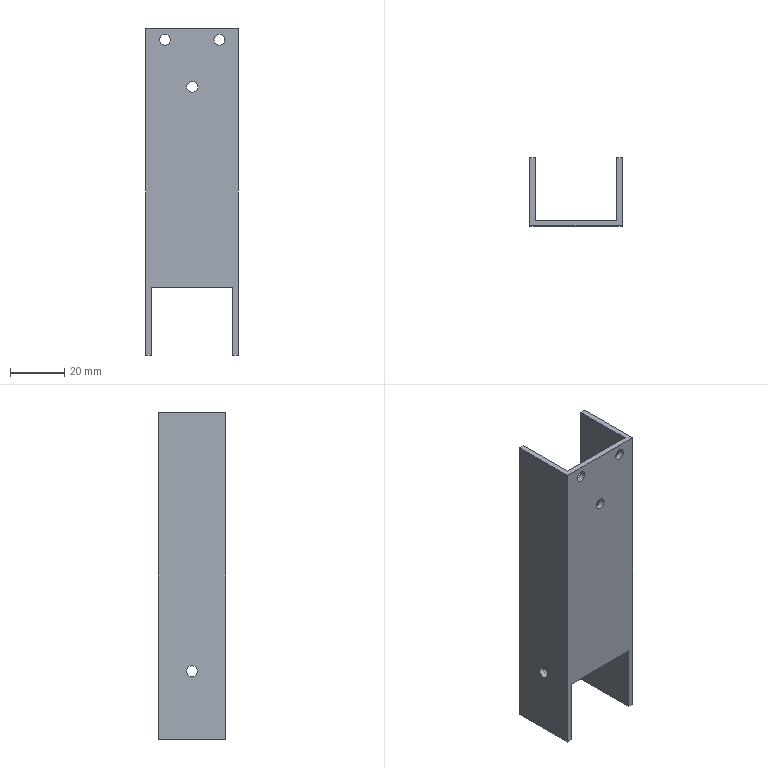Part | SolidWorks | features ICE 3, Extrusion 1 | 1 solid | 22 faces | box 34 x 25 x 120 mm | volume 17574 mm3 | plane 12 | cylinder 10 | commonest cylinder face diameters 4 x10
STEP:
#1=CARTESIAN_POINT('',(15.,8.5,25.));
#2=VERTEX_POINT('',#1);
#3=CARTESIAN_POINT('',(15.,12.5,25.));
#4=VERTEX_POINT('',#3);
#5=CARTESIAN_POINT('',(15.,10.5,25.));
#6=DIRECTION('',(1.,0.,0.));
#7=DIRECTION('',(0.,0.,-1.));
#8=AXIS2_PLACEMENT_3D('',#5,#6,#7);
#9=CIRCLE('',#8,2.);
#10=EDGE_CURVE('',#2,#4,#9,.T.);
#11=ORIENTED_EDGE('',*,*,#10,.F.);
#12=CARTESIAN_POINT('',(17.,8.5,25.));
#13=VERTEX_POINT('',#12);
#14=CARTESIAN_POINT('',(-17.,8.5,25.));
#15=DIRECTION('',(1.,0.,0.));
#16=VECTOR('',#15,1000.);
#17=LINE('',#14,#16);
#18=EDGE_CURVE('',#2,#13,#17,.T.);
#19=ORIENTED_EDGE('',*,*,#18,.T.);
#20=CARTESIAN_POINT('',(17.,12.5,25.));
#21=VERTEX_POINT('',#20);
#22=CARTESIAN_POINT('',(17.,10.5,25.));
#23=DIRECTION('',(1.,0.,0.));
#24=DIRECTION('',(0.,1.,0.));
#25=AXIS2_PLACEMENT_3D('',#22,#23,#24);
#26=CIRCLE('',#25,2.);
#27=EDGE_CURVE('',#13,#21,#26,.T.);
#28=ORIENTED_EDGE('',*,*,#27,.T.);
#29=CARTESIAN_POINT('',(-17.,12.5,25.));
#30=DIRECTION('',(1.,0.,0.));
#31=VECTOR('',#30,1000.);
#32=LINE('',#29,#31);
#33=EDGE_CURVE('',#4,#21,#32,.T.);
#34=ORIENTED_EDGE('',*,*,#33,.F.);
#35=EDGE_LOOP('',(#11,#19,#28,#34));
#36=FACE_OUTER_BOUND('',#35,.T.);
#37=CARTESIAN_POINT('',(-17.,10.5,25.));
#38=DIRECTION('',(1.,0.,0.));
#39=DIRECTION('',(0.,1.,0.));
#40=AXIS2_PLACEMENT_3D('',#37,#38,#39);
#41=CYLINDRICAL_SURFACE('',#40,2.);
#42=ADVANCED_FACE('',(#36),#41,.F.);
#43=CARTESIAN_POINT('',(-17.,8.5,25.));
#44=VERTEX_POINT('',#43);
#45=CARTESIAN_POINT('',(-17.,12.5,25.));
#46=VERTEX_POINT('',#45);
#47=CARTESIAN_POINT('',(-17.,10.5,25.));
#48=DIRECTION('',(1.,0.,0.));
#49=DIRECTION('',(0.,1.,0.));
#50=AXIS2_PLACEMENT_3D('',#47,#48,#49);
#51=CIRCLE('',#50,2.);
#52=EDGE_CURVE('',#44,#46,#51,.T.);
#53=ORIENTED_EDGE('',*,*,#52,.F.);
#54=CARTESIAN_POINT('',(-15.,8.5,25.));
#55=VERTEX_POINT('',#54);
#56=CARTESIAN_POINT('',(-17.,8.5,25.));
#57=DIRECTION('',(1.,0.,0.));
#58=VECTOR('',#57,1000.);
#59=LINE('',#56,#58);
#60=EDGE_CURVE('',#44,#55,#59,.T.);
#61=ORIENTED_EDGE('',*,*,#60,.T.);
#62=CARTESIAN_POINT('',(-15.,12.5,25.));
#63=VERTEX_POINT('',#62);
#64=CARTESIAN_POINT('',(-15.,10.5,25.));
#65=DIRECTION('',(-1.,0.,0.));
#66=DIRECTION('',(0.,-1.,0.));
#67=AXIS2_PLACEMENT_3D('',#64,#65,#66);
#68=CIRCLE('',#67,2.);
#69=EDGE_CURVE('',#63,#55,#68,.T.);
#70=ORIENTED_EDGE('',*,*,#69,.F.);
#71=CARTESIAN_POINT('',(-17.,12.5,25.));
#72=DIRECTION('',(1.,0.,0.));
#73=VECTOR('',#72,1000.);
#74=LINE('',#71,#73);
#75=EDGE_CURVE('',#46,#63,#74,.T.);
#76=ORIENTED_EDGE('',*,*,#75,.F.);
#77=EDGE_LOOP('',(#53,#61,#70,#76));
#78=FACE_OUTER_BOUND('',#77,.T.);
#79=CARTESIAN_POINT('',(-17.,10.5,25.));
#80=DIRECTION('',(1.,0.,0.));
#81=DIRECTION('',(0.,1.,0.));
#82=AXIS2_PLACEMENT_3D('',#79,#80,#81);
#83=CYLINDRICAL_SURFACE('',#82,2.);
#84=ADVANCED_FACE('',(#78),#83,.F.);
#85=CARTESIAN_POINT('',(-11.929,0.,116.));
#86=VERTEX_POINT('',#85);
#87=CARTESIAN_POINT('',(-7.929,0.,116.));
#88=VERTEX_POINT('',#87);
#89=CARTESIAN_POINT('',(-9.929,0.,116.));
#90=DIRECTION('',(0.,-1.,0.));
#91=DIRECTION('',(1.,0.,0.));
#92=AXIS2_PLACEMENT_3D('',#89,#90,#91);
#93=CIRCLE('',#92,2.);
#94=EDGE_CURVE('',#86,#88,#93,.T.);
#95=ORIENTED_EDGE('',*,*,#94,.F.);
#96=CARTESIAN_POINT('',(-11.929,-2.,116.));
#97=VERTEX_POINT('',#96);
#98=CARTESIAN_POINT('',(-11.929,23.,116.));
#99=DIRECTION('',(0.,-1.,0.));
#100=VECTOR('',#99,1000.);
#101=LINE('',#98,#100);
#102=EDGE_CURVE('',#86,#97,#101,.T.);
#103=ORIENTED_EDGE('',*,*,#102,.T.);
#104=CARTESIAN_POINT('',(-7.929,-2.,116.));
#105=VERTEX_POINT('',#104);
#106=CARTESIAN_POINT('',(-9.929,-2.,116.));
#107=DIRECTION('',(0.,-1.,0.));
#108=DIRECTION('',(1.,0.,0.));
#109=AXIS2_PLACEMENT_3D('',#106,#107,#108);
#110=CIRCLE('',#109,2.);
#111=EDGE_CURVE('',#97,#105,#110,.T.);
#112=ORIENTED_EDGE('',*,*,#111,.T.);
#113=CARTESIAN_POINT('',(-7.929,23.,116.));
#114=DIRECTION('',(0.,-1.,0.));
#115=VECTOR('',#114,1000.);
#116=LINE('',#113,#115);
#117=EDGE_CURVE('',#88,#105,#116,.T.);
#118=ORIENTED_EDGE('',*,*,#117,.F.);
#119=EDGE_LOOP('',(#95,#103,#112,#118));
#120=FACE_OUTER_BOUND('',#119,.T.);
#121=CARTESIAN_POINT('',(-9.929,23.,116.));
#122=DIRECTION('',(0.,-1.,0.));
#123=DIRECTION('',(1.,0.,0.));
#124=AXIS2_PLACEMENT_3D('',#121,#122,#123);
#125=CYLINDRICAL_SURFACE('',#124,2.);
#126=ADVANCED_FACE('',(#120),#125,.F.);
#127=CARTESIAN_POINT('',(8.071,0.,116.));
#128=VERTEX_POINT('',#127);
#129=CARTESIAN_POINT('',(12.071,0.,116.));
#130=VERTEX_POINT('',#129);
#131=CARTESIAN_POINT('',(10.071,0.,116.));
#132=DIRECTION('',(0.,-1.,0.));
#133=DIRECTION('',(1.,0.,0.));
#134=AXIS2_PLACEMENT_3D('',#131,#132,#133);
#135=CIRCLE('',#134,2.);
#136=EDGE_CURVE('',#128,#130,#135,.T.);
#137=ORIENTED_EDGE('',*,*,#136,.F.);
#138=CARTESIAN_POINT('',(8.071,-2.,116.));
#139=VERTEX_POINT('',#138);
#140=CARTESIAN_POINT('',(8.071,23.,116.));
#141=DIRECTION('',(0.,-1.,0.));
#142=VECTOR('',#141,1000.);
#143=LINE('',#140,#142);
#144=EDGE_CURVE('',#128,#139,#143,.T.);
#145=ORIENTED_EDGE('',*,*,#144,.T.);
#146=CARTESIAN_POINT('',(12.071,-2.,116.));
#147=VERTEX_POINT('',#146);
#148=CARTESIAN_POINT('',(10.071,-2.,116.));
#149=DIRECTION('',(0.,-1.,0.));
#150=DIRECTION('',(1.,0.,0.));
#151=AXIS2_PLACEMENT_3D('',#148,#149,#150);
#152=CIRCLE('',#151,2.);
#153=EDGE_CURVE('',#139,#147,#152,.T.);
#154=ORIENTED_EDGE('',*,*,#153,.T.);
#155=CARTESIAN_POINT('',(12.071,23.,116.));
#156=DIRECTION('',(0.,-1.,0.));
#157=VECTOR('',#156,1000.);
#158=LINE('',#155,#157);
#159=EDGE_CURVE('',#130,#147,#158,.T.);
#160=ORIENTED_EDGE('',*,*,#159,.F.);
#161=EDGE_LOOP('',(#137,#145,#154,#160));
#162=FACE_OUTER_BOUND('',#161,.T.);
#163=CARTESIAN_POINT('',(10.071,23.,116.));
#164=DIRECTION('',(0.,-1.,0.));
#165=DIRECTION('',(1.,0.,0.));
#166=AXIS2_PLACEMENT_3D('',#163,#164,#165);
#167=CYLINDRICAL_SURFACE('',#166,2.);
#168=ADVANCED_FACE('',(#162),#167,.F.);
#169=CARTESIAN_POINT('',(-1.929,0.,98.679));
#170=VERTEX_POINT('',#169);
#171=CARTESIAN_POINT('',(2.071,0.,98.679));
#172=VERTEX_POINT('',#171);
#173=CARTESIAN_POINT('',(0.07126,0.,98.679));
#174=DIRECTION('',(0.,-1.,0.));
#175=DIRECTION('',(1.,0.,0.));
#176=AXIS2_PLACEMENT_3D('',#173,#174,#175);
#177=CIRCLE('',#176,2.);
#178=EDGE_CURVE('',#170,#172,#177,.T.);
#179=ORIENTED_EDGE('',*,*,#178,.F.);
#180=CARTESIAN_POINT('',(-1.929,-2.,98.679));
#181=VERTEX_POINT('',#180);
#182=CARTESIAN_POINT('',(-1.929,23.,98.679));
#183=DIRECTION('',(0.,-1.,0.));
#184=VECTOR('',#183,1000.);
#185=LINE('',#182,#184);
#186=EDGE_CURVE('',#170,#181,#185,.T.);
#187=ORIENTED_EDGE('',*,*,#186,.T.);
#188=CARTESIAN_POINT('',(2.071,-2.,98.679));
#189=VERTEX_POINT('',#188);
#190=CARTESIAN_POINT('',(0.07126,-2.,98.679));
#191=DIRECTION('',(0.,-1.,0.));
#192=DIRECTION('',(1.,0.,0.));
#193=AXIS2_PLACEMENT_3D('',#190,#191,#192);
#194=CIRCLE('',#193,2.);
#195=EDGE_CURVE('',#181,#189,#194,.T.);
#196=ORIENTED_EDGE('',*,*,#195,.T.);
#197=CARTESIAN_POINT('',(2.071,23.,98.679));
#198=DIRECTION('',(0.,-1.,0.));
#199=VECTOR('',#198,1000.);
#200=LINE('',#197,#199);
#201=EDGE_CURVE('',#172,#189,#200,.T.);
#202=ORIENTED_EDGE('',*,*,#201,.F.);
#203=EDGE_LOOP('',(#179,#187,#196,#202));
#204=FACE_OUTER_BOUND('',#203,.T.);
#205=CARTESIAN_POINT('',(0.07126,23.,98.679));
#206=DIRECTION('',(0.,-1.,0.));
#207=DIRECTION('',(1.,0.,0.));
#208=AXIS2_PLACEMENT_3D('',#205,#206,#207);
#209=CYLINDRICAL_SURFACE('',#208,2.);
#210=ADVANCED_FACE('',(#204),#209,.F.);
#211=CARTESIAN_POINT('',(-15.,-2.,0.));
#212=VERTEX_POINT('',#211);
#213=CARTESIAN_POINT('',(-15.,23.,0.));
#214=VERTEX_POINT('',#213);
#215=CARTESIAN_POINT('',(-15.,23.,0.));
#216=DIRECTION('',(0.,1.,0.));
#217=VECTOR('',#216,1000.);
#218=LINE('',#215,#217);
#219=EDGE_CURVE('',#212,#214,#218,.T.);
#220=ORIENTED_EDGE('',*,*,#219,.F.);
#221=CARTESIAN_POINT('',(-17.,-2.,0.));
#222=VERTEX_POINT('',#221);
#223=CARTESIAN_POINT('',(17.,-2.,0.));
#224=DIRECTION('',(1.,0.,0.));
#225=VECTOR('',#224,1000.);
#226=LINE('',#223,#225);
#227=EDGE_CURVE('',#222,#212,#226,.T.);
#228=ORIENTED_EDGE('',*,*,#227,.F.);
#229=CARTESIAN_POINT('',(-17.,23.,0.));
#230=VERTEX_POINT('',#229);
#231=CARTESIAN_POINT('',(-17.,-2.,0.));
#232=DIRECTION('',(0.,-1.,0.));
#233=VECTOR('',#232,1000.);
#234=LINE('',#231,#233);
#235=EDGE_CURVE('',#230,#222,#234,.T.);
#236=ORIENTED_EDGE('',*,*,#235,.F.);
#237=CARTESIAN_POINT('',(-17.,23.,0.));
#238=DIRECTION('',(-1.,0.,0.));
#239=VECTOR('',#238,1000.);
#240=LINE('',#237,#239);
#241=EDGE_CURVE('',#214,#230,#240,.T.);
#242=ORIENTED_EDGE('',*,*,#241,.F.);
#243=EDGE_LOOP('',(#220,#228,#236,#242));
#244=FACE_OUTER_BOUND('',#243,.T.);
#245=CARTESIAN_POINT('',(0.,0.,0.));
#246=DIRECTION('',(0.,0.,-1.));
#247=DIRECTION('',(-1.,0.,0.));
#248=AXIS2_PLACEMENT_3D('',#245,#246,#247);
#249=PLANE('',#248);
#250=ADVANCED_FACE('',(#244),#249,.T.);
#251=ORIENTED_EDGE('',*,*,#241,.T.);
#252=CARTESIAN_POINT('',(-17.,23.,120.));
#253=VERTEX_POINT('',#252);
#254=CARTESIAN_POINT('',(-17.,23.,120.));
#255=DIRECTION('',(0.,0.,-1.));
#256=VECTOR('',#255,1000.);
#257=LINE('',#254,#256);
#258=EDGE_CURVE('',#253,#230,#257,.T.);
#259=ORIENTED_EDGE('',*,*,#258,.F.);
#260=CARTESIAN_POINT('',(-15.,23.,120.));
#261=VERTEX_POINT('',#260);
#262=CARTESIAN_POINT('',(-17.,23.,120.));
#263=DIRECTION('',(-1.,0.,0.));
#264=VECTOR('',#263,1000.);
#265=LINE('',#262,#264);
#266=EDGE_CURVE('',#261,#253,#265,.T.);
#267=ORIENTED_EDGE('',*,*,#266,.F.);
#268=CARTESIAN_POINT('',(-15.,23.,120.));
#269=DIRECTION('',(0.,0.,-1.));
#270=VECTOR('',#269,1000.);
#271=LINE('',#268,#270);
#272=EDGE_CURVE('',#261,#214,#271,.T.);
#273=ORIENTED_EDGE('',*,*,#272,.T.);
#274=EDGE_LOOP('',(#251,#259,#267,#273));
#275=FACE_OUTER_BOUND('',#274,.T.);
#276=CARTESIAN_POINT('',(-17.,23.,120.));
#277=DIRECTION('',(0.,-1.,0.));
#278=DIRECTION('',(0.,0.,-1.));
#279=AXIS2_PLACEMENT_3D('',#276,#277,#278);
#280=PLANE('',#279);
#281=ADVANCED_FACE('',(#275),#280,.F.);
#282=CARTESIAN_POINT('',(-17.,10.5,25.));
#283=DIRECTION('',(1.,0.,0.));
#284=DIRECTION('',(0.,1.,0.));
#285=AXIS2_PLACEMENT_3D('',#282,#283,#284);
#286=CIRCLE('',#285,2.);
#287=EDGE_CURVE('',#46,#44,#286,.T.);
#288=ORIENTED_EDGE('',*,*,#287,.T.);
#289=ORIENTED_EDGE('',*,*,#52,.T.);
#290=EDGE_LOOP('',(#288,#289));
#291=FACE_BOUND('',#290,.T.);
#292=ORIENTED_EDGE('',*,*,#235,.T.);
#293=CARTESIAN_POINT('',(-17.,-2.,120.));
#294=VERTEX_POINT('',#293);
#295=CARTESIAN_POINT('',(-17.,-2.,120.));
#296=DIRECTION('',(0.,0.,-1.));
#297=VECTOR('',#296,1000.);
#298=LINE('',#295,#297);
#299=EDGE_CURVE('',#294,#222,#298,.T.);
#300=ORIENTED_EDGE('',*,*,#299,.F.);
#301=CARTESIAN_POINT('',(-17.,-2.,120.));
#302=DIRECTION('',(0.,-1.,0.));
#303=VECTOR('',#302,1000.);
#304=LINE('',#301,#303);
#305=EDGE_CURVE('',#253,#294,#304,.T.);
#306=ORIENTED_EDGE('',*,*,#305,.F.);
#307=ORIENTED_EDGE('',*,*,#258,.T.);
#308=EDGE_LOOP('',(#292,#300,#306,#307));
#309=FACE_OUTER_BOUND('',#308,.T.);
#310=CARTESIAN_POINT('',(-17.,-2.,120.));
#311=DIRECTION('',(1.,0.,0.));
#312=DIRECTION('',(0.,0.,-1.));
#313=AXIS2_PLACEMENT_3D('',#310,#311,#312);
#314=PLANE('',#313);
#315=ADVANCED_FACE('',(#291,#309),#314,.F.);
#316=ORIENTED_EDGE('',*,*,#227,.T.);
#317=CARTESIAN_POINT('',(-15.,-2.,25.));
#318=VERTEX_POINT('',#317);
#319=CARTESIAN_POINT('',(-15.,-2.,0.));
#320=DIRECTION('',(0.,0.,1.));
#321=VECTOR('',#320,1000.);
#322=LINE('',#319,#321);
#323=EDGE_CURVE('',#212,#318,#322,.T.);
#324=ORIENTED_EDGE('',*,*,#323,.T.);
#325=CARTESIAN_POINT('',(15.,-2.,25.));
#326=VERTEX_POINT('',#325);
#327=CARTESIAN_POINT('',(-15.,-2.,25.));
#328=DIRECTION('',(1.,0.,0.));
#329=VECTOR('',#328,1000.);
#330=LINE('',#327,#329);
#331=EDGE_CURVE('',#318,#326,#330,.T.);
#332=ORIENTED_EDGE('',*,*,#331,.T.);
#333=CARTESIAN_POINT('',(15.,-2.,0.));
#334=VERTEX_POINT('',#333);
#335=CARTESIAN_POINT('',(15.,-2.,0.));
#336=DIRECTION('',(0.,0.,-1.));
#337=VECTOR('',#336,1000.);
#338=LINE('',#335,#337);
#339=EDGE_CURVE('',#326,#334,#338,.T.);
#340=ORIENTED_EDGE('',*,*,#339,.T.);
#341=CARTESIAN_POINT('',(17.,-2.,0.));
#342=VERTEX_POINT('',#341);
#343=CARTESIAN_POINT('',(17.,-2.,0.));
#344=DIRECTION('',(1.,0.,0.));
#345=VECTOR('',#344,1000.);
#346=LINE('',#343,#345);
#347=EDGE_CURVE('',#334,#342,#346,.T.);
#348=ORIENTED_EDGE('',*,*,#347,.T.);
#349=CARTESIAN_POINT('',(17.,-2.,120.));
#350=VERTEX_POINT('',#349);
#351=CARTESIAN_POINT('',(17.,-2.,120.));
#352=DIRECTION('',(0.,0.,-1.));
#353=VECTOR('',#352,1000.);
#354=LINE('',#351,#353);
#355=EDGE_CURVE('',#350,#342,#354,.T.);
#356=ORIENTED_EDGE('',*,*,#355,.F.);
#357=CARTESIAN_POINT('',(17.,-2.,120.));
#358=DIRECTION('',(1.,0.,0.));
#359=VECTOR('',#358,1000.);
#360=LINE('',#357,#359);
#361=EDGE_CURVE('',#294,#350,#360,.T.);
#362=ORIENTED_EDGE('',*,*,#361,.F.);
#363=ORIENTED_EDGE('',*,*,#299,.T.);
#364=EDGE_LOOP('',(#316,#324,#332,#340,#348,#356,#362,#363));
#365=FACE_OUTER_BOUND('',#364,.T.);
#366=CARTESIAN_POINT('',(-9.929,-2.,116.));
#367=DIRECTION('',(0.,-1.,0.));
#368=DIRECTION('',(1.,0.,0.));
#369=AXIS2_PLACEMENT_3D('',#366,#367,#368);
#370=CIRCLE('',#369,2.);
#371=EDGE_CURVE('',#105,#97,#370,.T.);
#372=ORIENTED_EDGE('',*,*,#371,.F.);
#373=ORIENTED_EDGE('',*,*,#111,.F.);
#374=EDGE_LOOP('',(#372,#373));
#375=FACE_BOUND('',#374,.T.);
#376=CARTESIAN_POINT('',(10.071,-2.,116.));
#377=DIRECTION('',(0.,-1.,0.));
#378=DIRECTION('',(1.,0.,0.));
#379=AXIS2_PLACEMENT_3D('',#376,#377,#378);
#380=CIRCLE('',#379,2.);
#381=EDGE_CURVE('',#147,#139,#380,.T.);
#382=ORIENTED_EDGE('',*,*,#381,.F.);
#383=ORIENTED_EDGE('',*,*,#153,.F.);
#384=EDGE_LOOP('',(#382,#383));
#385=FACE_BOUND('',#384,.T.);
#386=CARTESIAN_POINT('',(0.07126,-2.,98.679));
#387=DIRECTION('',(0.,-1.,0.));
#388=DIRECTION('',(1.,0.,0.));
#389=AXIS2_PLACEMENT_3D('',#386,#387,#388);
#390=CIRCLE('',#389,2.);
#391=EDGE_CURVE('',#189,#181,#390,.T.);
#392=ORIENTED_EDGE('',*,*,#391,.F.);
#393=ORIENTED_EDGE('',*,*,#195,.F.);
#394=EDGE_LOOP('',(#392,#393));
#395=FACE_BOUND('',#394,.T.);
#396=CARTESIAN_POINT('',(17.,-2.,120.));
#397=DIRECTION('',(0.,1.,0.));
#398=DIRECTION('',(-1.,0.,0.));
#399=AXIS2_PLACEMENT_3D('',#396,#397,#398);
#400=PLANE('',#399);
#401=ADVANCED_FACE('',(#365,#375,#385,#395),#400,.F.);
#402=CARTESIAN_POINT('',(17.,10.5,25.));
#403=DIRECTION('',(1.,0.,0.));
#404=DIRECTION('',(0.,1.,0.));
#405=AXIS2_PLACEMENT_3D('',#402,#403,#404);
#406=CIRCLE('',#405,2.);
#407=EDGE_CURVE('',#21,#13,#406,.T.);
#408=ORIENTED_EDGE('',*,*,#407,.F.);
#409=ORIENTED_EDGE('',*,*,#27,.F.);
#410=EDGE_LOOP('',(#408,#409));
#411=FACE_BOUND('',#410,.T.);
#412=CARTESIAN_POINT('',(17.,23.,0.));
#413=VERTEX_POINT('',#412);
#414=CARTESIAN_POINT('',(17.,23.,0.));
#415=DIRECTION('',(0.,1.,0.));
#416=VECTOR('',#415,1000.);
#417=LINE('',#414,#416);
#418=EDGE_CURVE('',#342,#413,#417,.T.);
#419=ORIENTED_EDGE('',*,*,#418,.T.);
#420=CARTESIAN_POINT('',(17.,23.,120.));
#421=VERTEX_POINT('',#420);
#422=CARTESIAN_POINT('',(17.,23.,120.));
#423=DIRECTION('',(0.,0.,-1.));
#424=VECTOR('',#423,1000.);
#425=LINE('',#422,#424);
#426=EDGE_CURVE('',#421,#413,#425,.T.);
#427=ORIENTED_EDGE('',*,*,#426,.F.);
#428=CARTESIAN_POINT('',(17.,23.,120.));
#429=DIRECTION('',(0.,1.,0.));
#430=VECTOR('',#429,1000.);
#431=LINE('',#428,#430);
#432=EDGE_CURVE('',#350,#421,#431,.T.);
#433=ORIENTED_EDGE('',*,*,#432,.F.);
#434=ORIENTED_EDGE('',*,*,#355,.T.);
#435=EDGE_LOOP('',(#419,#427,#433,#434));
#436=FACE_OUTER_BOUND('',#435,.T.);
#437=CARTESIAN_POINT('',(17.,23.,120.));
#438=DIRECTION('',(-1.,0.,0.));
#439=DIRECTION('',(0.,-1.,0.));
#440=AXIS2_PLACEMENT_3D('',#437,#438,#439);
#441=PLANE('',#440);
#442=ADVANCED_FACE('',(#411,#436),#441,.F.);
#443=CARTESIAN_POINT('',(15.,23.,0.));
#444=VERTEX_POINT('',#443);
#445=CARTESIAN_POINT('',(15.,23.,0.));
#446=DIRECTION('',(-1.,0.,0.));
#447=VECTOR('',#446,1000.);
#448=LINE('',#445,#447);
#449=EDGE_CURVE('',#413,#444,#448,.T.);
#450=ORIENTED_EDGE('',*,*,#449,.T.);
#451=CARTESIAN_POINT('',(15.,23.,120.));
#452=VERTEX_POINT('',#451);
#453=CARTESIAN_POINT('',(15.,23.,120.));
#454=DIRECTION('',(0.,0.,-1.));
#455=VECTOR('',#454,1000.);
#456=LINE('',#453,#455);
#457=EDGE_CURVE('',#452,#444,#456,.T.);
#458=ORIENTED_EDGE('',*,*,#457,.F.);
#459=CARTESIAN_POINT('',(15.,23.,120.));
#460=DIRECTION('',(-1.,0.,0.));
#461=VECTOR('',#460,1000.);
#462=LINE('',#459,#461);
#463=EDGE_CURVE('',#421,#452,#462,.T.);
#464=ORIENTED_EDGE('',*,*,#463,.F.);
#465=ORIENTED_EDGE('',*,*,#426,.T.);
#466=EDGE_LOOP('',(#450,#458,#464,#465));
#467=FACE_OUTER_BOUND('',#466,.T.);
#468=CARTESIAN_POINT('',(15.,23.,120.));
#469=DIRECTION('',(0.,-1.,0.));
#470=DIRECTION('',(0.,0.,-1.));
#471=AXIS2_PLACEMENT_3D('',#468,#469,#470);
#472=PLANE('',#471);
#473=ADVANCED_FACE('',(#467),#472,.F.);
#474=CARTESIAN_POINT('',(15.,10.5,25.));
#475=DIRECTION('',(1.,0.,0.));
#476=DIRECTION('',(0.,0.,-1.));
#477=AXIS2_PLACEMENT_3D('',#474,#475,#476);
#478=CIRCLE('',#477,2.);
#479=EDGE_CURVE('',#4,#2,#478,.T.);
#480=ORIENTED_EDGE('',*,*,#479,.T.);
#481=ORIENTED_EDGE('',*,*,#10,.T.);
#482=EDGE_LOOP('',(#480,#481));
#483=FACE_BOUND('',#482,.T.);
#484=CARTESIAN_POINT('',(15.,0.,0.));
#485=DIRECTION('',(0.,-1.,0.));
#486=VECTOR('',#485,1000.);
#487=LINE('',#484,#486);
#488=EDGE_CURVE('',#444,#334,#487,.T.);
#489=ORIENTED_EDGE('',*,*,#488,.T.);
#490=ORIENTED_EDGE('',*,*,#339,.F.);
#491=CARTESIAN_POINT('',(15.,0.,25.));
#492=VERTEX_POINT('',#491);
#493=CARTESIAN_POINT('',(15.,-2.,25.));
#494=DIRECTION('',(0.,1.,0.));
#495=VECTOR('',#494,1000.);
#496=LINE('',#493,#495);
#497=EDGE_CURVE('',#326,#492,#496,.T.);
#498=ORIENTED_EDGE('',*,*,#497,.T.);
#499=CARTESIAN_POINT('',(15.,0.,120.));
#500=VERTEX_POINT('',#499);
#501=CARTESIAN_POINT('',(15.,0.,120.));
#502=DIRECTION('',(0.,0.,-1.));
#503=VECTOR('',#502,1000.);
#504=LINE('',#501,#503);
#505=EDGE_CURVE('',#500,#492,#504,.T.);
#506=ORIENTED_EDGE('',*,*,#505,.F.);
#507=CARTESIAN_POINT('',(15.,0.,120.));
#508=DIRECTION('',(0.,-1.,0.));
#509=VECTOR('',#508,1000.);
#510=LINE('',#507,#509);
#511=EDGE_CURVE('',#452,#500,#510,.T.);
#512=ORIENTED_EDGE('',*,*,#511,.F.);
#513=ORIENTED_EDGE('',*,*,#457,.T.);
#514=EDGE_LOOP('',(#489,#490,#498,#506,#512,#513));
#515=FACE_OUTER_BOUND('',#514,.T.);
#516=CARTESIAN_POINT('',(15.,0.,120.));
#517=DIRECTION('',(1.,0.,0.));
#518=DIRECTION('',(0.,0.,-1.));
#519=AXIS2_PLACEMENT_3D('',#516,#517,#518);
#520=PLANE('',#519);
#521=ADVANCED_FACE('',(#483,#515),#520,.F.);
#522=CARTESIAN_POINT('',(-9.929,0.,116.));
#523=DIRECTION('',(0.,-1.,0.));
#524=DIRECTION('',(1.,0.,0.));
#525=AXIS2_PLACEMENT_3D('',#522,#523,#524);
#526=CIRCLE('',#525,2.);
#527=EDGE_CURVE('',#88,#86,#526,.T.);
#528=ORIENTED_EDGE('',*,*,#527,.T.);
#529=ORIENTED_EDGE('',*,*,#94,.T.);
#530=EDGE_LOOP('',(#528,#529));
#531=FACE_BOUND('',#530,.T.);
#532=CARTESIAN_POINT('',(10.071,0.,116.));
#533=DIRECTION('',(0.,-1.,0.));
#534=DIRECTION('',(1.,0.,0.));
#535=AXIS2_PLACEMENT_3D('',#532,#533,#534);
#536=CIRCLE('',#535,2.);
#537=EDGE_CURVE('',#130,#128,#536,.T.);
#538=ORIENTED_EDGE('',*,*,#537,.T.);
#539=ORIENTED_EDGE('',*,*,#136,.T.);
#540=EDGE_LOOP('',(#538,#539));
#541=FACE_BOUND('',#540,.T.);
#542=CARTESIAN_POINT('',(0.07126,0.,98.679));
#543=DIRECTION('',(0.,-1.,0.));
#544=DIRECTION('',(1.,0.,0.));
#545=AXIS2_PLACEMENT_3D('',#542,#543,#544);
#546=CIRCLE('',#545,2.);
#547=EDGE_CURVE('',#172,#170,#546,.T.);
#548=ORIENTED_EDGE('',*,*,#547,.T.);
#549=ORIENTED_EDGE('',*,*,#178,.T.);
#550=EDGE_LOOP('',(#548,#549));
#551=FACE_BOUND('',#550,.T.);
#552=ORIENTED_EDGE('',*,*,#505,.T.);
#553=CARTESIAN_POINT('',(-15.,0.,25.));
#554=VERTEX_POINT('',#553);
#555=CARTESIAN_POINT('',(-15.,0.,25.));
#556=DIRECTION('',(1.,0.,0.));
#557=VECTOR('',#556,1000.);
#558=LINE('',#555,#557);
#559=EDGE_CURVE('',#554,#492,#558,.T.);
#560=ORIENTED_EDGE('',*,*,#559,.F.);
#561=CARTESIAN_POINT('',(-15.,0.,120.));
#562=VERTEX_POINT('',#561);
#563=CARTESIAN_POINT('',(-15.,0.,120.));
#564=DIRECTION('',(0.,0.,-1.));
#565=VECTOR('',#564,1000.);
#566=LINE('',#563,#565);
#567=EDGE_CURVE('',#562,#554,#566,.T.);
#568=ORIENTED_EDGE('',*,*,#567,.F.);
#569=CARTESIAN_POINT('',(-15.,0.,120.));
#570=DIRECTION('',(-1.,0.,0.));
#571=VECTOR('',#570,1000.);
#572=LINE('',#569,#571);
#573=EDGE_CURVE('',#500,#562,#572,.T.);
#574=ORIENTED_EDGE('',*,*,#573,.F.);
#575=EDGE_LOOP('',(#552,#560,#568,#574));
#576=FACE_OUTER_BOUND('',#575,.T.);
#577=CARTESIAN_POINT('',(-15.,0.,120.));
#578=DIRECTION('',(0.,-1.,0.));
#579=DIRECTION('',(1.,0.,0.));
#580=AXIS2_PLACEMENT_3D('',#577,#578,#579);
#581=PLANE('',#580);
#582=ADVANCED_FACE('',(#531,#541,#551,#576),#581,.F.);
#583=ORIENTED_EDGE('',*,*,#69,.T.);
#584=CARTESIAN_POINT('',(-15.,10.5,25.));
#585=DIRECTION('',(-1.,0.,0.));
#586=DIRECTION('',(0.,-1.,0.));
#587=AXIS2_PLACEMENT_3D('',#584,#585,#586);
#588=CIRCLE('',#587,2.);
#589=EDGE_CURVE('',#55,#63,#588,.T.);
#590=ORIENTED_EDGE('',*,*,#589,.T.);
#591=EDGE_LOOP('',(#583,#590));
#592=FACE_BOUND('',#591,.T.);
#593=ORIENTED_EDGE('',*,*,#219,.T.);
#594=ORIENTED_EDGE('',*,*,#272,.F.);
#595=CARTESIAN_POINT('',(-15.,23.,120.));
#596=DIRECTION('',(0.,1.,0.));
#597=VECTOR('',#596,1000.);
#598=LINE('',#595,#597);
#599=EDGE_CURVE('',#562,#261,#598,.T.);
#600=ORIENTED_EDGE('',*,*,#599,.F.);
#601=ORIENTED_EDGE('',*,*,#567,.T.);
#602=CARTESIAN_POINT('',(-15.,-2.,25.));
#603=DIRECTION('',(0.,1.,0.));
#604=VECTOR('',#603,1000.);
#605=LINE('',#602,#604);
#606=EDGE_CURVE('',#318,#554,#605,.T.);
#607=ORIENTED_EDGE('',*,*,#606,.F.);
#608=ORIENTED_EDGE('',*,*,#323,.F.);
#609=EDGE_LOOP('',(#593,#594,#600,#601,#607,#608));
#610=FACE_OUTER_BOUND('',#609,.T.);
#611=CARTESIAN_POINT('',(-15.,23.,120.));
#612=DIRECTION('',(-1.,0.,0.));
#613=DIRECTION('',(0.,-1.,0.));
#614=AXIS2_PLACEMENT_3D('',#611,#612,#613);
#615=PLANE('',#614);
#616=ADVANCED_FACE('',(#592,#610),#615,.F.);
#617=ORIENTED_EDGE('',*,*,#266,.T.);
#618=ORIENTED_EDGE('',*,*,#305,.T.);
#619=ORIENTED_EDGE('',*,*,#361,.T.);
#620=ORIENTED_EDGE('',*,*,#432,.T.);
#621=ORIENTED_EDGE('',*,*,#463,.T.);
#622=ORIENTED_EDGE('',*,*,#511,.T.);
#623=ORIENTED_EDGE('',*,*,#573,.T.);
#624=ORIENTED_EDGE('',*,*,#599,.T.);
#625=EDGE_LOOP('',(#617,#618,#619,#620,#621,#622,#623,#624));
#626=FACE_OUTER_BOUND('',#625,.T.);
#627=CARTESIAN_POINT('',(0.,0.,120.));
#628=DIRECTION('',(0.,0.,-1.));
#629=DIRECTION('',(-1.,0.,0.));
#630=AXIS2_PLACEMENT_3D('',#627,#628,#629);
#631=PLANE('',#630);
#632=ADVANCED_FACE('',(#626),#631,.F.);
#633=ORIENTED_EDGE('',*,*,#347,.F.);
#634=ORIENTED_EDGE('',*,*,#488,.F.);
#635=ORIENTED_EDGE('',*,*,#449,.F.);
#636=ORIENTED_EDGE('',*,*,#418,.F.);
#637=EDGE_LOOP('',(#633,#634,#635,#636));
#638=FACE_OUTER_BOUND('',#637,.T.);
#639=CARTESIAN_POINT('',(0.,0.,0.));
#640=DIRECTION('',(0.,0.,-1.));
#641=DIRECTION('',(-1.,0.,0.));
#642=AXIS2_PLACEMENT_3D('',#639,#640,#641);
#643=PLANE('',#642);
#644=ADVANCED_FACE('',(#638),#643,.T.);
#645=ORIENTED_EDGE('',*,*,#186,.F.);
#646=ORIENTED_EDGE('',*,*,#547,.F.);
#647=ORIENTED_EDGE('',*,*,#201,.T.);
#648=ORIENTED_EDGE('',*,*,#391,.T.);
#649=EDGE_LOOP('',(#645,#646,#647,#648));
#650=FACE_OUTER_BOUND('',#649,.T.);
#651=CARTESIAN_POINT('',(0.07126,23.,98.679));
#652=DIRECTION('',(0.,-1.,0.));
#653=DIRECTION('',(1.,0.,0.));
#654=AXIS2_PLACEMENT_3D('',#651,#652,#653);
#655=CYLINDRICAL_SURFACE('',#654,2.);
#656=ADVANCED_FACE('',(#650),#655,.F.);
#657=ORIENTED_EDGE('',*,*,#144,.F.);
#658=ORIENTED_EDGE('',*,*,#537,.F.);
#659=ORIENTED_EDGE('',*,*,#159,.T.);
#660=ORIENTED_EDGE('',*,*,#381,.T.);
#661=EDGE_LOOP('',(#657,#658,#659,#660));
#662=FACE_OUTER_BOUND('',#661,.T.);
#663=CARTESIAN_POINT('',(10.071,23.,116.));
#664=DIRECTION('',(0.,-1.,0.));
#665=DIRECTION('',(1.,0.,0.));
#666=AXIS2_PLACEMENT_3D('',#663,#664,#665);
#667=CYLINDRICAL_SURFACE('',#666,2.);
#668=ADVANCED_FACE('',(#662),#667,.F.);
#669=ORIENTED_EDGE('',*,*,#102,.F.);
#670=ORIENTED_EDGE('',*,*,#527,.F.);
#671=ORIENTED_EDGE('',*,*,#117,.T.);
#672=ORIENTED_EDGE('',*,*,#371,.T.);
#673=EDGE_LOOP('',(#669,#670,#671,#672));
#674=FACE_OUTER_BOUND('',#673,.T.);
#675=CARTESIAN_POINT('',(-9.929,23.,116.));
#676=DIRECTION('',(0.,-1.,0.));
#677=DIRECTION('',(1.,0.,0.));
#678=AXIS2_PLACEMENT_3D('',#675,#676,#677);
#679=CYLINDRICAL_SURFACE('',#678,2.);
#680=ADVANCED_FACE('',(#674),#679,.F.);
#681=ORIENTED_EDGE('',*,*,#559,.T.);
#682=ORIENTED_EDGE('',*,*,#497,.F.);
#683=ORIENTED_EDGE('',*,*,#331,.F.);
#684=ORIENTED_EDGE('',*,*,#606,.T.);
#685=EDGE_LOOP('',(#681,#682,#683,#684));
#686=FACE_OUTER_BOUND('',#685,.T.);
#687=CARTESIAN_POINT('',(-15.,-2.,25.));
#688=DIRECTION('',(0.,0.,1.));
#689=DIRECTION('',(1.,0.,0.));
#690=AXIS2_PLACEMENT_3D('',#687,#688,#689);
#691=PLANE('',#690);
#692=ADVANCED_FACE('',(#686),#691,.F.);
#693=ORIENTED_EDGE('',*,*,#60,.F.);
#694=ORIENTED_EDGE('',*,*,#287,.F.);
#695=ORIENTED_EDGE('',*,*,#75,.T.);
#696=ORIENTED_EDGE('',*,*,#589,.F.);
#697=EDGE_LOOP('',(#693,#694,#695,#696));
#698=FACE_OUTER_BOUND('',#697,.T.);
#699=CARTESIAN_POINT('',(-17.,10.5,25.));
#700=DIRECTION('',(1.,0.,0.));
#701=DIRECTION('',(0.,1.,0.));
#702=AXIS2_PLACEMENT_3D('',#699,#700,#701);
#703=CYLINDRICAL_SURFACE('',#702,2.);
#704=ADVANCED_FACE('',(#698),#703,.F.);
#705=ORIENTED_EDGE('',*,*,#18,.F.);
#706=ORIENTED_EDGE('',*,*,#479,.F.);
#707=ORIENTED_EDGE('',*,*,#33,.T.);
#708=ORIENTED_EDGE('',*,*,#407,.T.);
#709=EDGE_LOOP('',(#705,#706,#707,#708));
#710=FACE_OUTER_BOUND('',#709,.T.);
#711=CARTESIAN_POINT('',(-17.,10.5,25.));
#712=DIRECTION('',(1.,0.,0.));
#713=DIRECTION('',(0.,1.,0.));
#714=AXIS2_PLACEMENT_3D('',#711,#712,#713);
#715=CYLINDRICAL_SURFACE('',#714,2.);
#716=ADVANCED_FACE('',(#710),#715,.F.);
#717=CLOSED_SHELL('',(#42,#84,#126,#168,#210,#250,#281,#315,#401,#442,#473,#521,#582,#616,#632,#644,#656,#668,#680,#692,#704,#716));
#718=MANIFOLD_SOLID_BREP('',#717);
#719=CARTESIAN_POINT('',(0.,0.,0.));
#720=DIRECTION('',(0.,0.,1.));
#721=DIRECTION('',(1.,0.,0.));
#722=AXIS2_PLACEMENT_3D('',#719,#720,#721);
#723=(LENGTH_UNIT()NAMED_UNIT(*)SI_UNIT(.MILLI.,.METRE.));
#724=UNCERTAINTY_MEASURE_WITH_UNIT(LENGTH_MEASURE(0.00001),#723,'','');
#725=(NAMED_UNIT(*)PLANE_ANGLE_UNIT()SI_UNIT($,.RADIAN.));
#726=(NAMED_UNIT(*)SI_UNIT($,.STERADIAN.)SOLID_ANGLE_UNIT());
#727=(GEOMETRIC_REPRESENTATION_CONTEXT(3)GLOBAL_UNCERTAINTY_ASSIGNED_CONTEXT((#724))GLOBAL_UNIT_ASSIGNED_CONTEXT((#723,#725,#726))REPRESENTATION_CONTEXT('',''));
#728=ADVANCED_BREP_SHAPE_REPRESENTATION('',(#718,#722),#727);